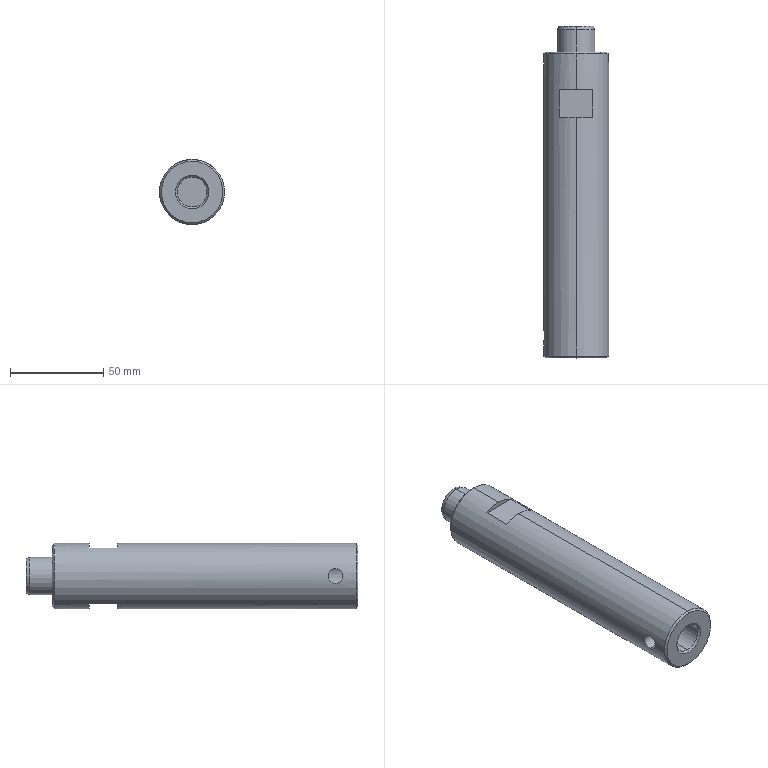Part | STEP file | OP10-106_guide post | 1 solid | 29 faces | box 35 x 178 x 35 mm | volume 152676 mm3 | plane 11 | cylinder 10 | cone 8 | commonest cylinder face diameters 8 x2 12 x2 16 x2 20 x2 35 x2